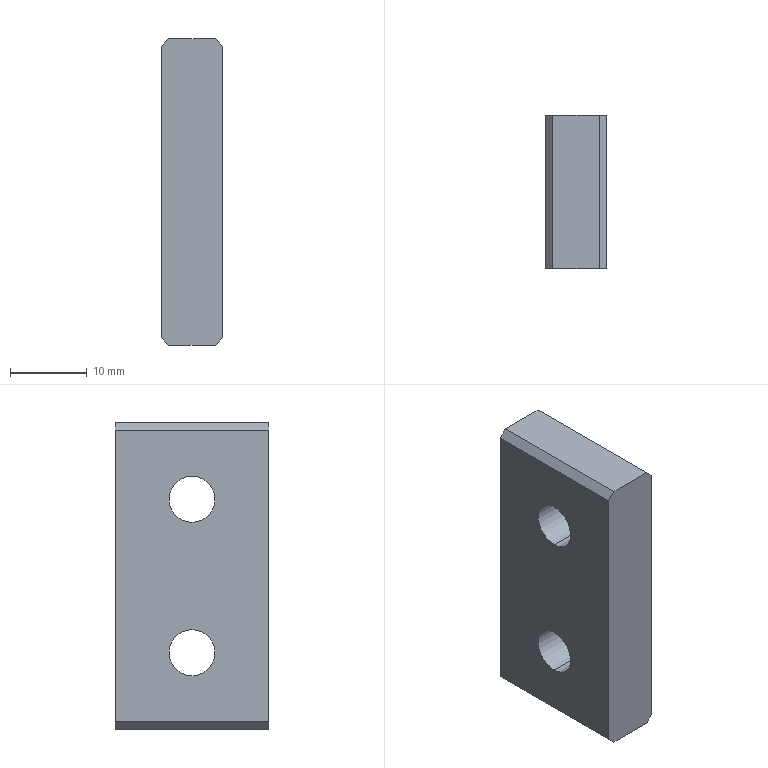Part | SolidWorks | features Chamfer 1, Extrusion 1, ICE 1 | 1 solid | 14 faces | box 8 x 20 x 40 mm | volume 5908 mm3 | plane 10 | cylinder 4 | commonest cylinder face diameters 6 x4
STEP:
#1=CARTESIAN_POINT('',(0.,10.,33.));
#2=VERTEX_POINT('',#1);
#3=CARTESIAN_POINT('',(0.,10.,27.));
#4=VERTEX_POINT('',#3);
#5=CARTESIAN_POINT('',(0.,10.,30.));
#6=DIRECTION('',(1.,0.,0.));
#7=DIRECTION('',(0.,0.,-1.));
#8=AXIS2_PLACEMENT_3D('',#5,#6,#7);
#9=CIRCLE('',#8,3.);
#10=EDGE_CURVE('',#2,#4,#9,.T.);
#11=ORIENTED_EDGE('',*,*,#10,.F.);
#12=CARTESIAN_POINT('',(8.,10.,33.));
#13=VERTEX_POINT('',#12);
#14=CARTESIAN_POINT('',(0.,10.,33.));
#15=DIRECTION('',(1.,0.,0.));
#16=VECTOR('',#15,1000.);
#17=LINE('',#14,#16);
#18=EDGE_CURVE('',#2,#13,#17,.T.);
#19=ORIENTED_EDGE('',*,*,#18,.T.);
#20=CARTESIAN_POINT('',(8.,10.,27.));
#21=VERTEX_POINT('',#20);
#22=CARTESIAN_POINT('',(8.,10.,30.));
#23=DIRECTION('',(1.,0.,0.));
#24=DIRECTION('',(0.,0.,-1.));
#25=AXIS2_PLACEMENT_3D('',#22,#23,#24);
#26=CIRCLE('',#25,3.);
#27=EDGE_CURVE('',#13,#21,#26,.T.);
#28=ORIENTED_EDGE('',*,*,#27,.T.);
#29=CARTESIAN_POINT('',(0.,10.,27.));
#30=DIRECTION('',(1.,0.,0.));
#31=VECTOR('',#30,1000.);
#32=LINE('',#29,#31);
#33=EDGE_CURVE('',#4,#21,#32,.T.);
#34=ORIENTED_EDGE('',*,*,#33,.F.);
#35=EDGE_LOOP('',(#11,#19,#28,#34));
#36=FACE_OUTER_BOUND('',#35,.T.);
#37=CARTESIAN_POINT('',(0.,10.,30.));
#38=DIRECTION('',(1.,0.,0.));
#39=DIRECTION('',(0.,0.,-1.));
#40=AXIS2_PLACEMENT_3D('',#37,#38,#39);
#41=CYLINDRICAL_SURFACE('',#40,3.);
#42=ADVANCED_FACE('',(#36),#41,.F.);
#43=CARTESIAN_POINT('',(0.,10.,13.));
#44=VERTEX_POINT('',#43);
#45=CARTESIAN_POINT('',(0.,10.,7.));
#46=VERTEX_POINT('',#45);
#47=CARTESIAN_POINT('',(0.,10.,10.));
#48=DIRECTION('',(1.,0.,0.));
#49=DIRECTION('',(0.,0.,-1.));
#50=AXIS2_PLACEMENT_3D('',#47,#48,#49);
#51=CIRCLE('',#50,3.);
#52=EDGE_CURVE('',#44,#46,#51,.T.);
#53=ORIENTED_EDGE('',*,*,#52,.F.);
#54=CARTESIAN_POINT('',(8.,10.,13.));
#55=VERTEX_POINT('',#54);
#56=CARTESIAN_POINT('',(0.,10.,13.));
#57=DIRECTION('',(1.,0.,0.));
#58=VECTOR('',#57,1000.);
#59=LINE('',#56,#58);
#60=EDGE_CURVE('',#44,#55,#59,.T.);
#61=ORIENTED_EDGE('',*,*,#60,.T.);
#62=CARTESIAN_POINT('',(8.,10.,7.));
#63=VERTEX_POINT('',#62);
#64=CARTESIAN_POINT('',(8.,10.,10.));
#65=DIRECTION('',(1.,0.,0.));
#66=DIRECTION('',(0.,0.,-1.));
#67=AXIS2_PLACEMENT_3D('',#64,#65,#66);
#68=CIRCLE('',#67,3.);
#69=EDGE_CURVE('',#55,#63,#68,.T.);
#70=ORIENTED_EDGE('',*,*,#69,.T.);
#71=CARTESIAN_POINT('',(0.,10.,7.));
#72=DIRECTION('',(1.,0.,0.));
#73=VECTOR('',#72,1000.);
#74=LINE('',#71,#73);
#75=EDGE_CURVE('',#46,#63,#74,.T.);
#76=ORIENTED_EDGE('',*,*,#75,.F.);
#77=EDGE_LOOP('',(#53,#61,#70,#76));
#78=FACE_OUTER_BOUND('',#77,.T.);
#79=CARTESIAN_POINT('',(0.,10.,10.));
#80=DIRECTION('',(1.,0.,0.));
#81=DIRECTION('',(0.,0.,-1.));
#82=AXIS2_PLACEMENT_3D('',#79,#80,#81);
#83=CYLINDRICAL_SURFACE('',#82,3.);
#84=ADVANCED_FACE('',(#78),#83,.F.);
#85=CARTESIAN_POINT('',(0.,10.,30.));
#86=DIRECTION('',(1.,0.,0.));
#87=DIRECTION('',(0.,0.,-1.));
#88=AXIS2_PLACEMENT_3D('',#85,#86,#87);
#89=CIRCLE('',#88,3.);
#90=EDGE_CURVE('',#4,#2,#89,.T.);
#91=ORIENTED_EDGE('',*,*,#90,.T.);
#92=ORIENTED_EDGE('',*,*,#10,.T.);
#93=EDGE_LOOP('',(#91,#92));
#94=FACE_BOUND('',#93,.T.);
#95=CARTESIAN_POINT('',(0.,10.,10.));
#96=DIRECTION('',(1.,0.,0.));
#97=DIRECTION('',(0.,0.,-1.));
#98=AXIS2_PLACEMENT_3D('',#95,#96,#97);
#99=CIRCLE('',#98,3.);
#100=EDGE_CURVE('',#46,#44,#99,.T.);
#101=ORIENTED_EDGE('',*,*,#100,.T.);
#102=ORIENTED_EDGE('',*,*,#52,.T.);
#103=EDGE_LOOP('',(#101,#102));
#104=FACE_BOUND('',#103,.T.);
#105=CARTESIAN_POINT('',(0.,20.,1.));
#106=VERTEX_POINT('',#105);
#107=CARTESIAN_POINT('',(0.,20.,39.));
#108=VERTEX_POINT('',#107);
#109=CARTESIAN_POINT('',(0.,20.,0.));
#110=DIRECTION('',(0.,0.,1.));
#111=VECTOR('',#110,1000.);
#112=LINE('',#109,#111);
#113=EDGE_CURVE('',#106,#108,#112,.T.);
#114=ORIENTED_EDGE('',*,*,#113,.F.);
#115=CARTESIAN_POINT('',(0.,0.,1.));
#116=VERTEX_POINT('',#115);
#117=CARTESIAN_POINT('',(0.,20.,1.));
#118=DIRECTION('',(0.,-1.,0.));
#119=VECTOR('',#118,1000.);
#120=LINE('',#117,#119);
#121=EDGE_CURVE('',#106,#116,#120,.T.);
#122=ORIENTED_EDGE('',*,*,#121,.T.);
#123=CARTESIAN_POINT('',(0.,0.,39.));
#124=VERTEX_POINT('',#123);
#125=CARTESIAN_POINT('',(0.,0.,0.));
#126=DIRECTION('',(0.,0.,1.));
#127=VECTOR('',#126,1000.);
#128=LINE('',#125,#127);
#129=EDGE_CURVE('',#116,#124,#128,.T.);
#130=ORIENTED_EDGE('',*,*,#129,.T.);
#131=CARTESIAN_POINT('',(0.,20.,39.));
#132=DIRECTION('',(0.,1.,0.));
#133=VECTOR('',#132,1000.);
#134=LINE('',#131,#133);
#135=EDGE_CURVE('',#124,#108,#134,.T.);
#136=ORIENTED_EDGE('',*,*,#135,.T.);
#137=EDGE_LOOP('',(#114,#122,#130,#136));
#138=FACE_OUTER_BOUND('',#137,.T.);
#139=CARTESIAN_POINT('',(0.,20.,0.));
#140=DIRECTION('',(1.,0.,0.));
#141=DIRECTION('',(0.,0.,-1.));
#142=AXIS2_PLACEMENT_3D('',#139,#140,#141);
#143=PLANE('',#142);
#144=ADVANCED_FACE('',(#94,#104,#138),#143,.F.);
#145=CARTESIAN_POINT('',(1.,20.,40.));
#146=VERTEX_POINT('',#145);
#147=CARTESIAN_POINT('',(7.,20.,40.));
#148=VERTEX_POINT('',#147);
#149=CARTESIAN_POINT('',(0.,20.,40.));
#150=DIRECTION('',(1.,0.,0.));
#151=VECTOR('',#150,1000.);
#152=LINE('',#149,#151);
#153=EDGE_CURVE('',#146,#148,#152,.T.);
#154=ORIENTED_EDGE('',*,*,#153,.F.);
#155=CARTESIAN_POINT('',(1.,0.,40.));
#156=VERTEX_POINT('',#155);
#157=CARTESIAN_POINT('',(1.,20.,40.));
#158=DIRECTION('',(0.,-1.,0.));
#159=VECTOR('',#158,1000.);
#160=LINE('',#157,#159);
#161=EDGE_CURVE('',#146,#156,#160,.T.);
#162=ORIENTED_EDGE('',*,*,#161,.T.);
#163=CARTESIAN_POINT('',(7.,0.,40.));
#164=VERTEX_POINT('',#163);
#165=CARTESIAN_POINT('',(0.,0.,40.));
#166=DIRECTION('',(1.,0.,0.));
#167=VECTOR('',#166,1000.);
#168=LINE('',#165,#167);
#169=EDGE_CURVE('',#156,#164,#168,.T.);
#170=ORIENTED_EDGE('',*,*,#169,.T.);
#171=CARTESIAN_POINT('',(7.,20.,40.));
#172=DIRECTION('',(0.,1.,0.));
#173=VECTOR('',#172,1000.);
#174=LINE('',#171,#173);
#175=EDGE_CURVE('',#164,#148,#174,.T.);
#176=ORIENTED_EDGE('',*,*,#175,.T.);
#177=EDGE_LOOP('',(#154,#162,#170,#176));
#178=FACE_OUTER_BOUND('',#177,.T.);
#179=CARTESIAN_POINT('',(0.,20.,40.));
#180=DIRECTION('',(0.,0.,-1.));
#181=DIRECTION('',(-1.,0.,0.));
#182=AXIS2_PLACEMENT_3D('',#179,#180,#181);
#183=PLANE('',#182);
#184=ADVANCED_FACE('',(#178),#183,.F.);
#185=CARTESIAN_POINT('',(8.,10.,30.));
#186=DIRECTION('',(1.,0.,0.));
#187=DIRECTION('',(0.,0.,-1.));
#188=AXIS2_PLACEMENT_3D('',#185,#186,#187);
#189=CIRCLE('',#188,3.);
#190=EDGE_CURVE('',#21,#13,#189,.T.);
#191=ORIENTED_EDGE('',*,*,#190,.F.);
#192=ORIENTED_EDGE('',*,*,#27,.F.);
#193=EDGE_LOOP('',(#191,#192));
#194=FACE_BOUND('',#193,.T.);
#195=CARTESIAN_POINT('',(8.,10.,10.));
#196=DIRECTION('',(1.,0.,0.));
#197=DIRECTION('',(0.,0.,-1.));
#198=AXIS2_PLACEMENT_3D('',#195,#196,#197);
#199=CIRCLE('',#198,3.);
#200=EDGE_CURVE('',#63,#55,#199,.T.);
#201=ORIENTED_EDGE('',*,*,#200,.F.);
#202=ORIENTED_EDGE('',*,*,#69,.F.);
#203=EDGE_LOOP('',(#201,#202));
#204=FACE_BOUND('',#203,.T.);
#205=CARTESIAN_POINT('',(8.,0.,39.));
#206=VERTEX_POINT('',#205);
#207=CARTESIAN_POINT('',(8.,0.,1.));
#208=VERTEX_POINT('',#207);
#209=CARTESIAN_POINT('',(8.,0.,0.));
#210=DIRECTION('',(0.,0.,-1.));
#211=VECTOR('',#210,1000.);
#212=LINE('',#209,#211);
#213=EDGE_CURVE('',#206,#208,#212,.T.);
#214=ORIENTED_EDGE('',*,*,#213,.T.);
#215=CARTESIAN_POINT('',(8.,20.,1.));
#216=VERTEX_POINT('',#215);
#217=CARTESIAN_POINT('',(8.,20.,1.));
#218=DIRECTION('',(0.,1.,0.));
#219=VECTOR('',#218,1000.);
#220=LINE('',#217,#219);
#221=EDGE_CURVE('',#208,#216,#220,.T.);
#222=ORIENTED_EDGE('',*,*,#221,.T.);
#223=CARTESIAN_POINT('',(8.,20.,39.));
#224=VERTEX_POINT('',#223);
#225=CARTESIAN_POINT('',(8.,20.,0.));
#226=DIRECTION('',(0.,0.,-1.));
#227=VECTOR('',#226,1000.);
#228=LINE('',#225,#227);
#229=EDGE_CURVE('',#224,#216,#228,.T.);
#230=ORIENTED_EDGE('',*,*,#229,.F.);
#231=CARTESIAN_POINT('',(8.,20.,39.));
#232=DIRECTION('',(0.,-1.,0.));
#233=VECTOR('',#232,1000.);
#234=LINE('',#231,#233);
#235=EDGE_CURVE('',#224,#206,#234,.T.);
#236=ORIENTED_EDGE('',*,*,#235,.T.);
#237=EDGE_LOOP('',(#214,#222,#230,#236));
#238=FACE_OUTER_BOUND('',#237,.T.);
#239=CARTESIAN_POINT('',(8.,20.,0.));
#240=DIRECTION('',(-1.,0.,0.));
#241=DIRECTION('',(0.,0.,1.));
#242=AXIS2_PLACEMENT_3D('',#239,#240,#241);
#243=PLANE('',#242);
#244=ADVANCED_FACE('',(#194,#204,#238),#243,.F.);
#245=CARTESIAN_POINT('',(7.,0.,0.));
#246=VERTEX_POINT('',#245);
#247=CARTESIAN_POINT('',(1.,0.,0.));
#248=VERTEX_POINT('',#247);
#249=CARTESIAN_POINT('',(0.,0.,0.));
#250=DIRECTION('',(-1.,0.,0.));
#251=VECTOR('',#250,1000.);
#252=LINE('',#249,#251);
#253=EDGE_CURVE('',#246,#248,#252,.T.);
#254=ORIENTED_EDGE('',*,*,#253,.T.);
#255=CARTESIAN_POINT('',(1.,20.,0.));
#256=VERTEX_POINT('',#255);
#257=CARTESIAN_POINT('',(1.,20.,0.));
#258=DIRECTION('',(0.,1.,0.));
#259=VECTOR('',#258,1000.);
#260=LINE('',#257,#259);
#261=EDGE_CURVE('',#248,#256,#260,.T.);
#262=ORIENTED_EDGE('',*,*,#261,.T.);
#263=CARTESIAN_POINT('',(7.,20.,0.));
#264=VERTEX_POINT('',#263);
#265=CARTESIAN_POINT('',(0.,20.,0.));
#266=DIRECTION('',(-1.,0.,0.));
#267=VECTOR('',#266,1000.);
#268=LINE('',#265,#267);
#269=EDGE_CURVE('',#264,#256,#268,.T.);
#270=ORIENTED_EDGE('',*,*,#269,.F.);
#271=CARTESIAN_POINT('',(7.,20.,0.));
#272=DIRECTION('',(0.,-1.,0.));
#273=VECTOR('',#272,1000.);
#274=LINE('',#271,#273);
#275=EDGE_CURVE('',#264,#246,#274,.T.);
#276=ORIENTED_EDGE('',*,*,#275,.T.);
#277=EDGE_LOOP('',(#254,#262,#270,#276));
#278=FACE_OUTER_BOUND('',#277,.T.);
#279=CARTESIAN_POINT('',(0.,20.,0.));
#280=DIRECTION('',(0.,0.,1.));
#281=DIRECTION('',(1.,0.,0.));
#282=AXIS2_PLACEMENT_3D('',#279,#280,#281);
#283=PLANE('',#282);
#284=ADVANCED_FACE('',(#278),#283,.F.);
#285=ORIENTED_EDGE('',*,*,#269,.T.);
#286=CARTESIAN_POINT('',(0.5,20.,0.5));
#287=DIRECTION('',(-0.7071,0.,0.7071));
#288=VECTOR('',#287,1000.);
#289=LINE('',#286,#288);
#290=EDGE_CURVE('',#256,#106,#289,.T.);
#291=ORIENTED_EDGE('',*,*,#290,.T.);
#292=ORIENTED_EDGE('',*,*,#113,.T.);
#293=CARTESIAN_POINT('',(-19.5,20.,19.5));
#294=DIRECTION('',(0.7071,0.,0.7071));
#295=VECTOR('',#294,1000.);
#296=LINE('',#293,#295);
#297=EDGE_CURVE('',#108,#146,#296,.T.);
#298=ORIENTED_EDGE('',*,*,#297,.T.);
#299=ORIENTED_EDGE('',*,*,#153,.T.);
#300=CARTESIAN_POINT('',(23.5,20.,23.5));
#301=DIRECTION('',(0.7071,0.,-0.7071));
#302=VECTOR('',#301,1000.);
#303=LINE('',#300,#302);
#304=EDGE_CURVE('',#148,#224,#303,.T.);
#305=ORIENTED_EDGE('',*,*,#304,.T.);
#306=ORIENTED_EDGE('',*,*,#229,.T.);
#307=CARTESIAN_POINT('',(3.5,20.,-3.5));
#308=DIRECTION('',(-0.7071,0.,-0.7071));
#309=VECTOR('',#308,1000.);
#310=LINE('',#307,#309);
#311=EDGE_CURVE('',#216,#264,#310,.T.);
#312=ORIENTED_EDGE('',*,*,#311,.T.);
#313=EDGE_LOOP('',(#285,#291,#292,#298,#299,#305,#306,#312));
#314=FACE_OUTER_BOUND('',#313,.T.);
#315=CARTESIAN_POINT('',(0.,20.,0.));
#316=DIRECTION('',(0.,1.,0.));
#317=DIRECTION('',(0.,0.,1.));
#318=AXIS2_PLACEMENT_3D('',#315,#316,#317);
#319=PLANE('',#318);
#320=ADVANCED_FACE('',(#314),#319,.T.);
#321=ORIENTED_EDGE('',*,*,#129,.F.);
#322=CARTESIAN_POINT('',(0.,0.,1.));
#323=DIRECTION('',(0.7071,0.,-0.7071));
#324=VECTOR('',#323,1000.);
#325=LINE('',#322,#324);
#326=EDGE_CURVE('',#116,#248,#325,.T.);
#327=ORIENTED_EDGE('',*,*,#326,.T.);
#328=ORIENTED_EDGE('',*,*,#253,.F.);
#329=CARTESIAN_POINT('',(7.,0.,0.));
#330=DIRECTION('',(0.7071,0.,0.7071));
#331=VECTOR('',#330,1000.);
#332=LINE('',#329,#331);
#333=EDGE_CURVE('',#246,#208,#332,.T.);
#334=ORIENTED_EDGE('',*,*,#333,.T.);
#335=ORIENTED_EDGE('',*,*,#213,.F.);
#336=CARTESIAN_POINT('',(8.,0.,39.));
#337=DIRECTION('',(-0.7071,0.,0.7071));
#338=VECTOR('',#337,1000.);
#339=LINE('',#336,#338);
#340=EDGE_CURVE('',#206,#164,#339,.T.);
#341=ORIENTED_EDGE('',*,*,#340,.T.);
#342=ORIENTED_EDGE('',*,*,#169,.F.);
#343=CARTESIAN_POINT('',(1.,0.,40.));
#344=DIRECTION('',(-0.7071,0.,-0.7071));
#345=VECTOR('',#344,1000.);
#346=LINE('',#343,#345);
#347=EDGE_CURVE('',#156,#124,#346,.T.);
#348=ORIENTED_EDGE('',*,*,#347,.T.);
#349=EDGE_LOOP('',(#321,#327,#328,#334,#335,#341,#342,#348));
#350=FACE_OUTER_BOUND('',#349,.T.);
#351=CARTESIAN_POINT('',(0.,0.,0.));
#352=DIRECTION('',(0.,1.,0.));
#353=DIRECTION('',(0.,0.,1.));
#354=AXIS2_PLACEMENT_3D('',#351,#352,#353);
#355=PLANE('',#354);
#356=ADVANCED_FACE('',(#350),#355,.F.);
#357=ORIENTED_EDGE('',*,*,#290,.F.);
#358=ORIENTED_EDGE('',*,*,#261,.F.);
#359=ORIENTED_EDGE('',*,*,#326,.F.);
#360=ORIENTED_EDGE('',*,*,#121,.F.);
#361=EDGE_LOOP('',(#357,#358,#359,#360));
#362=FACE_OUTER_BOUND('',#361,.T.);
#363=CARTESIAN_POINT('',(0.,20.,1.));
#364=DIRECTION('',(0.7071,0.,0.7071));
#365=DIRECTION('',(0.,-1.,0.));
#366=AXIS2_PLACEMENT_3D('',#363,#364,#365);
#367=PLANE('',#366);
#368=ADVANCED_FACE('',(#362),#367,.F.);
#369=ORIENTED_EDGE('',*,*,#311,.F.);
#370=ORIENTED_EDGE('',*,*,#221,.F.);
#371=ORIENTED_EDGE('',*,*,#333,.F.);
#372=ORIENTED_EDGE('',*,*,#275,.F.);
#373=EDGE_LOOP('',(#369,#370,#371,#372));
#374=FACE_OUTER_BOUND('',#373,.T.);
#375=CARTESIAN_POINT('',(7.,20.,0.));
#376=DIRECTION('',(-0.7071,0.,0.7071));
#377=DIRECTION('',(0.,-1.,0.));
#378=AXIS2_PLACEMENT_3D('',#375,#376,#377);
#379=PLANE('',#378);
#380=ADVANCED_FACE('',(#374),#379,.F.);
#381=ORIENTED_EDGE('',*,*,#297,.F.);
#382=ORIENTED_EDGE('',*,*,#135,.F.);
#383=ORIENTED_EDGE('',*,*,#347,.F.);
#384=ORIENTED_EDGE('',*,*,#161,.F.);
#385=EDGE_LOOP('',(#381,#382,#383,#384));
#386=FACE_OUTER_BOUND('',#385,.T.);
#387=CARTESIAN_POINT('',(1.,20.,40.));
#388=DIRECTION('',(0.7071,0.,-0.7071));
#389=DIRECTION('',(0.,-1.,0.));
#390=AXIS2_PLACEMENT_3D('',#387,#388,#389);
#391=PLANE('',#390);
#392=ADVANCED_FACE('',(#386),#391,.F.);
#393=ORIENTED_EDGE('',*,*,#304,.F.);
#394=ORIENTED_EDGE('',*,*,#175,.F.);
#395=ORIENTED_EDGE('',*,*,#340,.F.);
#396=ORIENTED_EDGE('',*,*,#235,.F.);
#397=EDGE_LOOP('',(#393,#394,#395,#396));
#398=FACE_OUTER_BOUND('',#397,.T.);
#399=CARTESIAN_POINT('',(8.,20.,39.));
#400=DIRECTION('',(-0.7071,0.,-0.7071));
#401=DIRECTION('',(0.,-1.,0.));
#402=AXIS2_PLACEMENT_3D('',#399,#400,#401);
#403=PLANE('',#402);
#404=ADVANCED_FACE('',(#398),#403,.F.);
#405=ORIENTED_EDGE('',*,*,#60,.F.);
#406=ORIENTED_EDGE('',*,*,#100,.F.);
#407=ORIENTED_EDGE('',*,*,#75,.T.);
#408=ORIENTED_EDGE('',*,*,#200,.T.);
#409=EDGE_LOOP('',(#405,#406,#407,#408));
#410=FACE_OUTER_BOUND('',#409,.T.);
#411=CARTESIAN_POINT('',(0.,10.,10.));
#412=DIRECTION('',(1.,0.,0.));
#413=DIRECTION('',(0.,0.,-1.));
#414=AXIS2_PLACEMENT_3D('',#411,#412,#413);
#415=CYLINDRICAL_SURFACE('',#414,3.);
#416=ADVANCED_FACE('',(#410),#415,.F.);
#417=ORIENTED_EDGE('',*,*,#18,.F.);
#418=ORIENTED_EDGE('',*,*,#90,.F.);
#419=ORIENTED_EDGE('',*,*,#33,.T.);
#420=ORIENTED_EDGE('',*,*,#190,.T.);
#421=EDGE_LOOP('',(#417,#418,#419,#420));
#422=FACE_OUTER_BOUND('',#421,.T.);
#423=CARTESIAN_POINT('',(0.,10.,30.));
#424=DIRECTION('',(1.,0.,0.));
#425=DIRECTION('',(0.,0.,-1.));
#426=AXIS2_PLACEMENT_3D('',#423,#424,#425);
#427=CYLINDRICAL_SURFACE('',#426,3.);
#428=ADVANCED_FACE('',(#422),#427,.F.);
#429=CLOSED_SHELL('',(#42,#84,#144,#184,#244,#284,#320,#356,#368,#380,#392,#404,#416,#428));
#430=MANIFOLD_SOLID_BREP('',#429);
#431=CARTESIAN_POINT('',(0.,0.,0.));
#432=DIRECTION('',(0.,0.,1.));
#433=DIRECTION('',(1.,0.,0.));
#434=AXIS2_PLACEMENT_3D('',#431,#432,#433);
#435=(LENGTH_UNIT()NAMED_UNIT(*)SI_UNIT(.MILLI.,.METRE.));
#436=UNCERTAINTY_MEASURE_WITH_UNIT(LENGTH_MEASURE(0.00001),#435,'','');
#437=(NAMED_UNIT(*)PLANE_ANGLE_UNIT()SI_UNIT($,.RADIAN.));
#438=(NAMED_UNIT(*)SI_UNIT($,.STERADIAN.)SOLID_ANGLE_UNIT());
#439=(GEOMETRIC_REPRESENTATION_CONTEXT(3)GLOBAL_UNCERTAINTY_ASSIGNED_CONTEXT((#436))GLOBAL_UNIT_ASSIGNED_CONTEXT((#435,#437,#438))REPRESENTATION_CONTEXT('',''));
#440=ADVANCED_BREP_SHAPE_REPRESENTATION('',(#430,#434),#439);